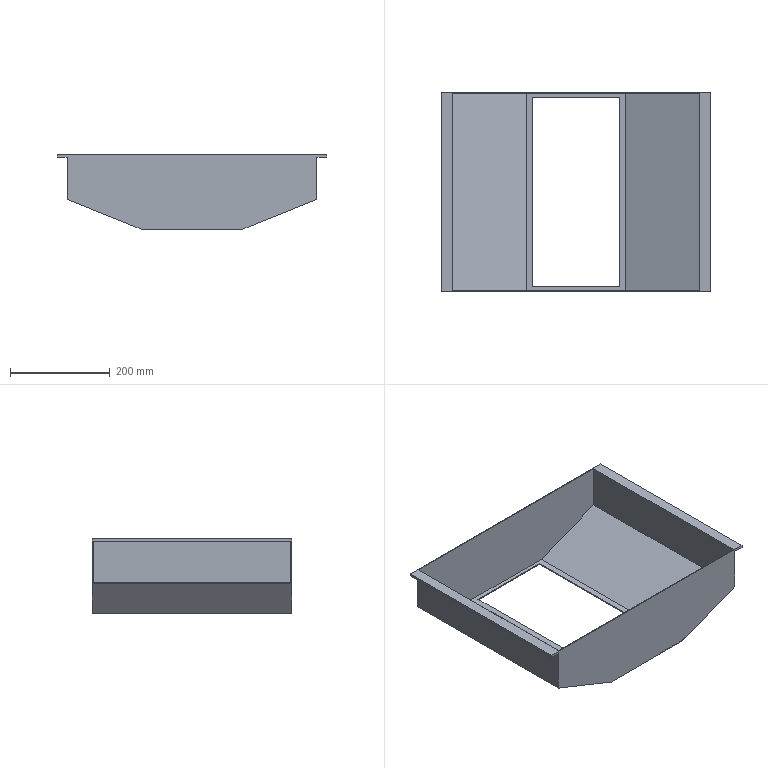Part | SolidWorks | features ICE 3, Extrusion 1, Shell 1 | 1 solid | 23 faces | box 540 x 400 x 150 mm | volume 765108 mm3 | plane 23
STEP:
#1=CARTESIAN_POINT('',(-99.615,198.,2.));
#2=VERTEX_POINT('',#1);
#3=CARTESIAN_POINT('',(-99.615,-198.,2.));
#4=VERTEX_POINT('',#3);
#5=CARTESIAN_POINT('',(-99.615,0.,2.));
#6=DIRECTION('',(0.,-1.,0.));
#7=VECTOR('',#6,1000.);
#8=LINE('',#5,#7);
#9=EDGE_CURVE('',#2,#4,#8,.T.);
#10=ORIENTED_EDGE('',*,*,#9,.T.);
#11=CARTESIAN_POINT('',(99.615,-198.,2.));
#12=VERTEX_POINT('',#11);
#13=CARTESIAN_POINT('',(0.,-198.,2.));
#14=DIRECTION('',(1.,0.,0.));
#15=VECTOR('',#14,1000.);
#16=LINE('',#13,#15);
#17=EDGE_CURVE('',#4,#12,#16,.T.);
#18=ORIENTED_EDGE('',*,*,#17,.T.);
#19=CARTESIAN_POINT('',(99.615,198.,2.));
#20=VERTEX_POINT('',#19);
#21=CARTESIAN_POINT('',(99.615,200.,2.));
#22=DIRECTION('',(0.,-1.,0.));
#23=VECTOR('',#22,1000.);
#24=LINE('',#21,#23);
#25=EDGE_CURVE('',#20,#12,#24,.T.);
#26=ORIENTED_EDGE('',*,*,#25,.F.);
#27=CARTESIAN_POINT('',(0.,198.,2.));
#28=DIRECTION('',(-1.,0.,0.));
#29=VECTOR('',#28,1000.);
#30=LINE('',#27,#29);
#31=EDGE_CURVE('',#20,#2,#30,.T.);
#32=ORIENTED_EDGE('',*,*,#31,.T.);
#33=EDGE_LOOP('',(#10,#18,#26,#32));
#34=FACE_OUTER_BOUND('',#33,.T.);
#35=CARTESIAN_POINT('',(87.5,-190.,2.));
#36=VERTEX_POINT('',#35);
#37=CARTESIAN_POINT('',(87.5,190.,2.));
#38=VERTEX_POINT('',#37);
#39=CARTESIAN_POINT('',(87.5,-190.,2.));
#40=DIRECTION('',(0.,1.,0.));
#41=VECTOR('',#40,1000.);
#42=LINE('',#39,#41);
#43=EDGE_CURVE('',#36,#38,#42,.T.);
#44=ORIENTED_EDGE('',*,*,#43,.F.);
#45=CARTESIAN_POINT('',(-87.5,-190.,2.));
#46=VERTEX_POINT('',#45);
#47=CARTESIAN_POINT('',(-87.5,-190.,2.));
#48=DIRECTION('',(1.,0.,0.));
#49=VECTOR('',#48,1000.);
#50=LINE('',#47,#49);
#51=EDGE_CURVE('',#46,#36,#50,.T.);
#52=ORIENTED_EDGE('',*,*,#51,.F.);
#53=CARTESIAN_POINT('',(-87.5,190.,2.));
#54=VERTEX_POINT('',#53);
#55=CARTESIAN_POINT('',(-87.5,-190.,2.));
#56=DIRECTION('',(0.,-1.,0.));
#57=VECTOR('',#56,1000.);
#58=LINE('',#55,#57);
#59=EDGE_CURVE('',#54,#46,#58,.T.);
#60=ORIENTED_EDGE('',*,*,#59,.F.);
#61=CARTESIAN_POINT('',(-87.5,190.,2.));
#62=DIRECTION('',(-1.,0.,0.));
#63=VECTOR('',#62,1000.);
#64=LINE('',#61,#63);
#65=EDGE_CURVE('',#38,#54,#64,.T.);
#66=ORIENTED_EDGE('',*,*,#65,.F.);
#67=EDGE_LOOP('',(#44,#52,#60,#66));
#68=FACE_BOUND('',#67,.T.);
#69=CARTESIAN_POINT('',(0.,0.,2.));
#70=DIRECTION('',(0.,0.,-1.));
#71=DIRECTION('',(-1.,0.,0.));
#72=AXIS2_PLACEMENT_3D('',#69,#70,#71);
#73=PLANE('',#72);
#74=ADVANCED_FACE('',(#34,#68),#73,.F.);
#75=CARTESIAN_POINT('',(-270.,-200.,150.));
#76=VERTEX_POINT('',#75);
#77=CARTESIAN_POINT('',(270.,-200.,150.));
#78=VERTEX_POINT('',#77);
#79=CARTESIAN_POINT('',(-250.,-200.,150.));
#80=DIRECTION('',(1.,0.,0.));
#81=VECTOR('',#80,1000.);
#82=LINE('',#79,#81);
#83=EDGE_CURVE('',#76,#78,#82,.T.);
#84=ORIENTED_EDGE('',*,*,#83,.T.);
#85=CARTESIAN_POINT('',(270.,200.,150.));
#86=VERTEX_POINT('',#85);
#87=CARTESIAN_POINT('',(270.,200.,150.));
#88=DIRECTION('',(0.,1.,0.));
#89=VECTOR('',#88,1000.);
#90=LINE('',#87,#89);
#91=EDGE_CURVE('',#78,#86,#90,.T.);
#92=ORIENTED_EDGE('',*,*,#91,.T.);
#93=CARTESIAN_POINT('',(-270.,200.,150.));
#94=VERTEX_POINT('',#93);
#95=CARTESIAN_POINT('',(-250.,200.,150.));
#96=DIRECTION('',(-1.,0.,0.));
#97=VECTOR('',#96,1000.);
#98=LINE('',#95,#97);
#99=EDGE_CURVE('',#86,#94,#98,.T.);
#100=ORIENTED_EDGE('',*,*,#99,.T.);
#101=CARTESIAN_POINT('',(-270.,200.,150.));
#102=DIRECTION('',(0.,-1.,0.));
#103=VECTOR('',#102,1000.);
#104=LINE('',#101,#103);
#105=EDGE_CURVE('',#94,#76,#104,.T.);
#106=ORIENTED_EDGE('',*,*,#105,.T.);
#107=EDGE_LOOP('',(#84,#92,#100,#106));
#108=FACE_OUTER_BOUND('',#107,.T.);
#109=CARTESIAN_POINT('',(248.,-198.,150.));
#110=VERTEX_POINT('',#109);
#111=CARTESIAN_POINT('',(248.,198.,150.));
#112=VERTEX_POINT('',#111);
#113=CARTESIAN_POINT('',(248.,0.,150.));
#114=DIRECTION('',(0.,1.,0.));
#115=VECTOR('',#114,1000.);
#116=LINE('',#113,#115);
#117=EDGE_CURVE('',#110,#112,#116,.T.);
#118=ORIENTED_EDGE('',*,*,#117,.F.);
#119=CARTESIAN_POINT('',(-248.,-198.,150.));
#120=VERTEX_POINT('',#119);
#121=CARTESIAN_POINT('',(0.,-198.,150.));
#122=DIRECTION('',(1.,0.,0.));
#123=VECTOR('',#122,1000.);
#124=LINE('',#121,#123);
#125=EDGE_CURVE('',#120,#110,#124,.T.);
#126=ORIENTED_EDGE('',*,*,#125,.F.);
#127=CARTESIAN_POINT('',(-248.,198.,150.));
#128=VERTEX_POINT('',#127);
#129=CARTESIAN_POINT('',(-248.,0.,150.));
#130=DIRECTION('',(0.,-1.,0.));
#131=VECTOR('',#130,1000.);
#132=LINE('',#129,#131);
#133=EDGE_CURVE('',#128,#120,#132,.T.);
#134=ORIENTED_EDGE('',*,*,#133,.F.);
#135=CARTESIAN_POINT('',(0.,198.,150.));
#136=DIRECTION('',(-1.,0.,0.));
#137=VECTOR('',#136,1000.);
#138=LINE('',#135,#137);
#139=EDGE_CURVE('',#112,#128,#138,.T.);
#140=ORIENTED_EDGE('',*,*,#139,.F.);
#141=EDGE_LOOP('',(#118,#126,#134,#140));
#142=FACE_BOUND('',#141,.T.);
#143=CARTESIAN_POINT('',(0.,0.,150.));
#144=DIRECTION('',(0.,0.,-1.));
#145=DIRECTION('',(-1.,0.,0.));
#146=AXIS2_PLACEMENT_3D('',#143,#144,#145);
#147=PLANE('',#146);
#148=ADVANCED_FACE('',(#108,#142),#147,.F.);
#149=CARTESIAN_POINT('',(250.,200.,145.));
#150=VERTEX_POINT('',#149);
#151=CARTESIAN_POINT('',(250.,200.,60.));
#152=VERTEX_POINT('',#151);
#153=CARTESIAN_POINT('',(250.,200.,150.));
#154=DIRECTION('',(0.,0.,-1.));
#155=VECTOR('',#154,1000.);
#156=LINE('',#153,#155);
#157=EDGE_CURVE('',#150,#152,#156,.T.);
#158=ORIENTED_EDGE('',*,*,#157,.F.);
#159=CARTESIAN_POINT('',(250.,-200.,145.));
#160=VERTEX_POINT('',#159);
#161=CARTESIAN_POINT('',(250.,200.,145.));
#162=DIRECTION('',(0.,-1.,0.));
#163=VECTOR('',#162,1000.);
#164=LINE('',#161,#163);
#165=EDGE_CURVE('',#150,#160,#164,.T.);
#166=ORIENTED_EDGE('',*,*,#165,.T.);
#167=CARTESIAN_POINT('',(250.,-200.,60.));
#168=VERTEX_POINT('',#167);
#169=CARTESIAN_POINT('',(250.,-200.,150.));
#170=DIRECTION('',(0.,0.,-1.));
#171=VECTOR('',#170,1000.);
#172=LINE('',#169,#171);
#173=EDGE_CURVE('',#160,#168,#172,.T.);
#174=ORIENTED_EDGE('',*,*,#173,.T.);
#175=CARTESIAN_POINT('',(250.,200.,60.));
#176=DIRECTION('',(0.,-1.,0.));
#177=VECTOR('',#176,1000.);
#178=LINE('',#175,#177);
#179=EDGE_CURVE('',#152,#168,#178,.T.);
#180=ORIENTED_EDGE('',*,*,#179,.F.);
#181=EDGE_LOOP('',(#158,#166,#174,#180));
#182=FACE_OUTER_BOUND('',#181,.T.);
#183=CARTESIAN_POINT('',(250.,-200.,150.));
#184=DIRECTION('',(-1.,0.,0.));
#185=DIRECTION('',(0.,0.,1.));
#186=AXIS2_PLACEMENT_3D('',#183,#184,#185);
#187=PLANE('',#186);
#188=ADVANCED_FACE('',(#182),#187,.F.);
#189=CARTESIAN_POINT('',(100.,200.,0.));
#190=VERTEX_POINT('',#189);
#191=CARTESIAN_POINT('',(-100.,200.,0.));
#192=VERTEX_POINT('',#191);
#193=CARTESIAN_POINT('',(-250.,200.,0.));
#194=DIRECTION('',(-1.,0.,0.));
#195=VECTOR('',#194,1000.);
#196=LINE('',#193,#195);
#197=EDGE_CURVE('',#190,#192,#196,.T.);
#198=ORIENTED_EDGE('',*,*,#197,.T.);
#199=CARTESIAN_POINT('',(-250.,200.,60.));
#200=VERTEX_POINT('',#199);
#201=CARTESIAN_POINT('',(-100.,200.,0.));
#202=DIRECTION('',(-0.9285,0.,0.3714));
#203=VECTOR('',#202,1000.);
#204=LINE('',#201,#203);
#205=EDGE_CURVE('',#192,#200,#204,.T.);
#206=ORIENTED_EDGE('',*,*,#205,.T.);
#207=CARTESIAN_POINT('',(-250.,200.,145.));
#208=VERTEX_POINT('',#207);
#209=CARTESIAN_POINT('',(-250.,200.,150.));
#210=DIRECTION('',(0.,0.,-1.));
#211=VECTOR('',#210,1000.);
#212=LINE('',#209,#211);
#213=EDGE_CURVE('',#208,#200,#212,.T.);
#214=ORIENTED_EDGE('',*,*,#213,.F.);
#215=CARTESIAN_POINT('',(-270.,200.,145.));
#216=VERTEX_POINT('',#215);
#217=CARTESIAN_POINT('',(-250.,200.,145.));
#218=DIRECTION('',(-1.,0.,0.));
#219=VECTOR('',#218,1000.);
#220=LINE('',#217,#219);
#221=EDGE_CURVE('',#208,#216,#220,.T.);
#222=ORIENTED_EDGE('',*,*,#221,.T.);
#223=CARTESIAN_POINT('',(-270.,200.,145.));
#224=DIRECTION('',(0.,0.,1.));
#225=VECTOR('',#224,1000.);
#226=LINE('',#223,#225);
#227=EDGE_CURVE('',#216,#94,#226,.T.);
#228=ORIENTED_EDGE('',*,*,#227,.T.);
#229=ORIENTED_EDGE('',*,*,#99,.F.);
#230=CARTESIAN_POINT('',(270.,200.,145.));
#231=VERTEX_POINT('',#230);
#232=CARTESIAN_POINT('',(270.,200.,145.));
#233=DIRECTION('',(0.,0.,1.));
#234=VECTOR('',#233,1000.);
#235=LINE('',#232,#234);
#236=EDGE_CURVE('',#231,#86,#235,.T.);
#237=ORIENTED_EDGE('',*,*,#236,.F.);
#238=CARTESIAN_POINT('',(250.,200.,145.));
#239=DIRECTION('',(-1.,0.,0.));
#240=VECTOR('',#239,1000.);
#241=LINE('',#238,#240);
#242=EDGE_CURVE('',#231,#150,#241,.T.);
#243=ORIENTED_EDGE('',*,*,#242,.T.);
#244=ORIENTED_EDGE('',*,*,#157,.T.);
#245=CARTESIAN_POINT('',(250.,200.,60.));
#246=DIRECTION('',(-0.9285,0.,-0.3714));
#247=VECTOR('',#246,1000.);
#248=LINE('',#245,#247);
#249=EDGE_CURVE('',#152,#190,#248,.T.);
#250=ORIENTED_EDGE('',*,*,#249,.T.);
#251=EDGE_LOOP('',(#198,#206,#214,#222,#228,#229,#237,#243,#244,#250));
#252=FACE_OUTER_BOUND('',#251,.T.);
#253=CARTESIAN_POINT('',(-250.,200.,150.));
#254=DIRECTION('',(0.,-1.,0.));
#255=DIRECTION('',(0.,0.,-1.));
#256=AXIS2_PLACEMENT_3D('',#253,#254,#255);
#257=PLANE('',#256);
#258=ADVANCED_FACE('',(#252),#257,.F.);
#259=CARTESIAN_POINT('',(-250.,-200.,145.));
#260=VERTEX_POINT('',#259);
#261=CARTESIAN_POINT('',(-250.,-200.,60.));
#262=VERTEX_POINT('',#261);
#263=CARTESIAN_POINT('',(-250.,-200.,150.));
#264=DIRECTION('',(0.,0.,-1.));
#265=VECTOR('',#264,1000.);
#266=LINE('',#263,#265);
#267=EDGE_CURVE('',#260,#262,#266,.T.);
#268=ORIENTED_EDGE('',*,*,#267,.F.);
#269=CARTESIAN_POINT('',(-250.,200.,145.));
#270=DIRECTION('',(0.,1.,0.));
#271=VECTOR('',#270,1000.);
#272=LINE('',#269,#271);
#273=EDGE_CURVE('',#260,#208,#272,.T.);
#274=ORIENTED_EDGE('',*,*,#273,.T.);
#275=ORIENTED_EDGE('',*,*,#213,.T.);
#276=CARTESIAN_POINT('',(-250.,200.,60.));
#277=DIRECTION('',(0.,-1.,0.));
#278=VECTOR('',#277,1000.);
#279=LINE('',#276,#278);
#280=EDGE_CURVE('',#200,#262,#279,.T.);
#281=ORIENTED_EDGE('',*,*,#280,.T.);
#282=EDGE_LOOP('',(#268,#274,#275,#281));
#283=FACE_OUTER_BOUND('',#282,.T.);
#284=CARTESIAN_POINT('',(-250.,-200.,150.));
#285=DIRECTION('',(1.,0.,0.));
#286=DIRECTION('',(0.,0.,-1.));
#287=AXIS2_PLACEMENT_3D('',#284,#285,#286);
#288=PLANE('',#287);
#289=ADVANCED_FACE('',(#283),#288,.F.);
#290=ORIENTED_EDGE('',*,*,#83,.F.);
#291=CARTESIAN_POINT('',(-270.,-200.,145.));
#292=VERTEX_POINT('',#291);
#293=CARTESIAN_POINT('',(-270.,-200.,145.));
#294=DIRECTION('',(0.,0.,1.));
#295=VECTOR('',#294,1000.);
#296=LINE('',#293,#295);
#297=EDGE_CURVE('',#292,#76,#296,.T.);
#298=ORIENTED_EDGE('',*,*,#297,.F.);
#299=CARTESIAN_POINT('',(-250.,-200.,145.));
#300=DIRECTION('',(1.,0.,0.));
#301=VECTOR('',#300,1000.);
#302=LINE('',#299,#301);
#303=EDGE_CURVE('',#292,#260,#302,.T.);
#304=ORIENTED_EDGE('',*,*,#303,.T.);
#305=ORIENTED_EDGE('',*,*,#267,.T.);
#306=CARTESIAN_POINT('',(-100.,-200.,0.));
#307=VERTEX_POINT('',#306);
#308=CARTESIAN_POINT('',(-100.,-200.,0.));
#309=DIRECTION('',(-0.9285,0.,0.3714));
#310=VECTOR('',#309,1000.);
#311=LINE('',#308,#310);
#312=EDGE_CURVE('',#307,#262,#311,.T.);
#313=ORIENTED_EDGE('',*,*,#312,.F.);
#314=CARTESIAN_POINT('',(100.,-200.,0.));
#315=VERTEX_POINT('',#314);
#316=CARTESIAN_POINT('',(-250.,-200.,0.));
#317=DIRECTION('',(1.,0.,0.));
#318=VECTOR('',#317,1000.);
#319=LINE('',#316,#318);
#320=EDGE_CURVE('',#307,#315,#319,.T.);
#321=ORIENTED_EDGE('',*,*,#320,.T.);
#322=CARTESIAN_POINT('',(250.,-200.,60.));
#323=DIRECTION('',(-0.9285,0.,-0.3714));
#324=VECTOR('',#323,1000.);
#325=LINE('',#322,#324);
#326=EDGE_CURVE('',#168,#315,#325,.T.);
#327=ORIENTED_EDGE('',*,*,#326,.F.);
#328=ORIENTED_EDGE('',*,*,#173,.F.);
#329=CARTESIAN_POINT('',(270.,-200.,145.));
#330=VERTEX_POINT('',#329);
#331=CARTESIAN_POINT('',(250.,-200.,145.));
#332=DIRECTION('',(1.,0.,0.));
#333=VECTOR('',#332,1000.);
#334=LINE('',#331,#333);
#335=EDGE_CURVE('',#160,#330,#334,.T.);
#336=ORIENTED_EDGE('',*,*,#335,.T.);
#337=CARTESIAN_POINT('',(270.,-200.,145.));
#338=DIRECTION('',(0.,0.,1.));
#339=VECTOR('',#338,1000.);
#340=LINE('',#337,#339);
#341=EDGE_CURVE('',#330,#78,#340,.T.);
#342=ORIENTED_EDGE('',*,*,#341,.T.);
#343=EDGE_LOOP('',(#290,#298,#304,#305,#313,#321,#327,#328,#336,#342));
#344=FACE_OUTER_BOUND('',#343,.T.);
#345=CARTESIAN_POINT('',(-250.,-200.,150.));
#346=DIRECTION('',(0.,1.,0.));
#347=DIRECTION('',(0.,0.,1.));
#348=AXIS2_PLACEMENT_3D('',#345,#346,#347);
#349=PLANE('',#348);
#350=ADVANCED_FACE('',(#344),#349,.F.);
#351=CARTESIAN_POINT('',(87.5,-190.,0.));
#352=VERTEX_POINT('',#351);
#353=CARTESIAN_POINT('',(87.5,190.,0.));
#354=VERTEX_POINT('',#353);
#355=CARTESIAN_POINT('',(87.5,-190.,0.));
#356=DIRECTION('',(0.,1.,0.));
#357=VECTOR('',#356,1000.);
#358=LINE('',#355,#357);
#359=EDGE_CURVE('',#352,#354,#358,.T.);
#360=ORIENTED_EDGE('',*,*,#359,.T.);
#361=CARTESIAN_POINT('',(-87.5,190.,0.));
#362=VERTEX_POINT('',#361);
#363=CARTESIAN_POINT('',(-87.5,190.,0.));
#364=DIRECTION('',(-1.,0.,0.));
#365=VECTOR('',#364,1000.);
#366=LINE('',#363,#365);
#367=EDGE_CURVE('',#354,#362,#366,.T.);
#368=ORIENTED_EDGE('',*,*,#367,.T.);
#369=CARTESIAN_POINT('',(-87.5,-190.,0.));
#370=VERTEX_POINT('',#369);
#371=CARTESIAN_POINT('',(-87.5,-190.,0.));
#372=DIRECTION('',(0.,-1.,0.));
#373=VECTOR('',#372,1000.);
#374=LINE('',#371,#373);
#375=EDGE_CURVE('',#362,#370,#374,.T.);
#376=ORIENTED_EDGE('',*,*,#375,.T.);
#377=CARTESIAN_POINT('',(-87.5,-190.,0.));
#378=DIRECTION('',(1.,0.,0.));
#379=VECTOR('',#378,1000.);
#380=LINE('',#377,#379);
#381=EDGE_CURVE('',#370,#352,#380,.T.);
#382=ORIENTED_EDGE('',*,*,#381,.T.);
#383=EDGE_LOOP('',(#360,#368,#376,#382));
#384=FACE_BOUND('',#383,.T.);
#385=CARTESIAN_POINT('',(-100.,200.,0.));
#386=DIRECTION('',(0.,-1.,0.));
#387=VECTOR('',#386,1000.);
#388=LINE('',#385,#387);
#389=EDGE_CURVE('',#192,#307,#388,.T.);
#390=ORIENTED_EDGE('',*,*,#389,.F.);
#391=ORIENTED_EDGE('',*,*,#197,.F.);
#392=CARTESIAN_POINT('',(100.,200.,0.));
#393=DIRECTION('',(0.,-1.,0.));
#394=VECTOR('',#393,1000.);
#395=LINE('',#392,#394);
#396=EDGE_CURVE('',#190,#315,#395,.T.);
#397=ORIENTED_EDGE('',*,*,#396,.T.);
#398=ORIENTED_EDGE('',*,*,#320,.F.);
#399=EDGE_LOOP('',(#390,#391,#397,#398));
#400=FACE_OUTER_BOUND('',#399,.T.);
#401=CARTESIAN_POINT('',(0.,0.,0.));
#402=DIRECTION('',(0.,0.,-1.));
#403=DIRECTION('',(-1.,0.,0.));
#404=AXIS2_PLACEMENT_3D('',#401,#402,#403);
#405=PLANE('',#404);
#406=ADVANCED_FACE('',(#384,#400),#405,.T.);
#407=ORIENTED_EDGE('',*,*,#326,.T.);
#408=ORIENTED_EDGE('',*,*,#396,.F.);
#409=ORIENTED_EDGE('',*,*,#249,.F.);
#410=ORIENTED_EDGE('',*,*,#179,.T.);
#411=EDGE_LOOP('',(#407,#408,#409,#410));
#412=FACE_OUTER_BOUND('',#411,.T.);
#413=CARTESIAN_POINT('',(250.,200.,60.));
#414=DIRECTION('',(-0.3714,0.,0.9285));
#415=DIRECTION('',(0.9285,0.,0.3714));
#416=AXIS2_PLACEMENT_3D('',#413,#414,#415);
#417=PLANE('',#416);
#418=ADVANCED_FACE('',(#412),#417,.F.);
#419=ORIENTED_EDGE('',*,*,#312,.T.);
#420=ORIENTED_EDGE('',*,*,#280,.F.);
#421=ORIENTED_EDGE('',*,*,#205,.F.);
#422=ORIENTED_EDGE('',*,*,#389,.T.);
#423=EDGE_LOOP('',(#419,#420,#421,#422));
#424=FACE_OUTER_BOUND('',#423,.T.);
#425=CARTESIAN_POINT('',(-100.,200.,0.));
#426=DIRECTION('',(0.3714,0.,0.9285));
#427=DIRECTION('',(0.9285,0.,-0.3714));
#428=AXIS2_PLACEMENT_3D('',#425,#426,#427);
#429=PLANE('',#428);
#430=ADVANCED_FACE('',(#424),#429,.F.);
#431=CARTESIAN_POINT('',(248.,-198.,61.354));
#432=VERTEX_POINT('',#431);
#433=CARTESIAN_POINT('',(248.,-198.,150.));
#434=DIRECTION('',(0.,0.,-1.));
#435=VECTOR('',#434,1000.);
#436=LINE('',#433,#435);
#437=EDGE_CURVE('',#110,#432,#436,.T.);
#438=ORIENTED_EDGE('',*,*,#437,.F.);
#439=ORIENTED_EDGE('',*,*,#117,.T.);
#440=CARTESIAN_POINT('',(248.,198.,61.354));
#441=VERTEX_POINT('',#440);
#442=CARTESIAN_POINT('',(248.,198.,150.));
#443=DIRECTION('',(0.,0.,-1.));
#444=VECTOR('',#443,1000.);
#445=LINE('',#442,#444);
#446=EDGE_CURVE('',#112,#441,#445,.T.);
#447=ORIENTED_EDGE('',*,*,#446,.T.);
#448=CARTESIAN_POINT('',(248.,200.,61.354));
#449=DIRECTION('',(0.,-1.,0.));
#450=VECTOR('',#449,1000.);
#451=LINE('',#448,#450);
#452=EDGE_CURVE('',#441,#432,#451,.T.);
#453=ORIENTED_EDGE('',*,*,#452,.T.);
#454=EDGE_LOOP('',(#438,#439,#447,#453));
#455=FACE_OUTER_BOUND('',#454,.T.);
#456=CARTESIAN_POINT('',(248.,-200.,150.));
#457=DIRECTION('',(-1.,0.,0.));
#458=DIRECTION('',(0.,0.,1.));
#459=AXIS2_PLACEMENT_3D('',#456,#457,#458);
#460=PLANE('',#459);
#461=ADVANCED_FACE('',(#455),#460,.T.);
#462=ORIENTED_EDGE('',*,*,#31,.F.);
#463=CARTESIAN_POINT('',(-150.743,198.,-98.143));
#464=DIRECTION('',(-0.9285,0.,-0.3714));
#465=VECTOR('',#464,1000.);
#466=LINE('',#463,#465);
#467=EDGE_CURVE('',#441,#20,#466,.T.);
#468=ORIENTED_EDGE('',*,*,#467,.F.);
#469=ORIENTED_EDGE('',*,*,#446,.F.);
#470=ORIENTED_EDGE('',*,*,#139,.T.);
#471=CARTESIAN_POINT('',(-248.,198.,61.354));
#472=VERTEX_POINT('',#471);
#473=CARTESIAN_POINT('',(-248.,198.,150.));
#474=DIRECTION('',(0.,0.,-1.));
#475=VECTOR('',#474,1000.);
#476=LINE('',#473,#475);
#477=EDGE_CURVE('',#128,#472,#476,.T.);
#478=ORIENTED_EDGE('',*,*,#477,.T.);
#479=CARTESIAN_POINT('',(-280.292,198.,74.271));
#480=DIRECTION('',(-0.9285,0.,0.3714));
#481=VECTOR('',#480,1000.);
#482=LINE('',#479,#481);
#483=EDGE_CURVE('',#2,#472,#482,.T.);
#484=ORIENTED_EDGE('',*,*,#483,.F.);
#485=EDGE_LOOP('',(#462,#468,#469,#470,#478,#484));
#486=FACE_OUTER_BOUND('',#485,.T.);
#487=CARTESIAN_POINT('',(-250.,198.,150.));
#488=DIRECTION('',(0.,-1.,0.));
#489=DIRECTION('',(0.,0.,-1.));
#490=AXIS2_PLACEMENT_3D('',#487,#488,#489);
#491=PLANE('',#490);
#492=ADVANCED_FACE('',(#486),#491,.T.);
#493=ORIENTED_EDGE('',*,*,#477,.F.);
#494=ORIENTED_EDGE('',*,*,#133,.T.);
#495=CARTESIAN_POINT('',(-248.,-198.,61.354));
#496=VERTEX_POINT('',#495);
#497=CARTESIAN_POINT('',(-248.,-198.,150.));
#498=DIRECTION('',(0.,0.,-1.));
#499=VECTOR('',#498,1000.);
#500=LINE('',#497,#499);
#501=EDGE_CURVE('',#120,#496,#500,.T.);
#502=ORIENTED_EDGE('',*,*,#501,.T.);
#503=CARTESIAN_POINT('',(-248.,-200.,61.354));
#504=DIRECTION('',(0.,-1.,0.));
#505=VECTOR('',#504,1000.);
#506=LINE('',#503,#505);
#507=EDGE_CURVE('',#472,#496,#506,.T.);
#508=ORIENTED_EDGE('',*,*,#507,.F.);
#509=EDGE_LOOP('',(#493,#494,#502,#508));
#510=FACE_OUTER_BOUND('',#509,.T.);
#511=CARTESIAN_POINT('',(-248.,-200.,150.));
#512=DIRECTION('',(1.,0.,0.));
#513=DIRECTION('',(0.,0.,-1.));
#514=AXIS2_PLACEMENT_3D('',#511,#512,#513);
#515=PLANE('',#514);
#516=ADVANCED_FACE('',(#510),#515,.T.);
#517=ORIENTED_EDGE('',*,*,#501,.F.);
#518=ORIENTED_EDGE('',*,*,#125,.T.);
#519=ORIENTED_EDGE('',*,*,#437,.T.);
#520=CARTESIAN_POINT('',(249.257,-198.,61.857));
#521=DIRECTION('',(-0.9285,0.,-0.3714));
#522=VECTOR('',#521,1000.);
#523=LINE('',#520,#522);
#524=EDGE_CURVE('',#432,#12,#523,.T.);
#525=ORIENTED_EDGE('',*,*,#524,.T.);
#526=ORIENTED_EDGE('',*,*,#17,.F.);
#527=CARTESIAN_POINT('',(-99.257,-198.,1.857));
#528=DIRECTION('',(-0.9285,0.,0.3714));
#529=VECTOR('',#528,1000.);
#530=LINE('',#527,#529);
#531=EDGE_CURVE('',#4,#496,#530,.T.);
#532=ORIENTED_EDGE('',*,*,#531,.T.);
#533=EDGE_LOOP('',(#517,#518,#519,#525,#526,#532));
#534=FACE_OUTER_BOUND('',#533,.T.);
#535=CARTESIAN_POINT('',(-250.,-198.,150.));
#536=DIRECTION('',(0.,1.,0.));
#537=DIRECTION('',(0.,0.,1.));
#538=AXIS2_PLACEMENT_3D('',#535,#536,#537);
#539=PLANE('',#538);
#540=ADVANCED_FACE('',(#534),#539,.T.);
#541=ORIENTED_EDGE('',*,*,#524,.F.);
#542=ORIENTED_EDGE('',*,*,#452,.F.);
#543=ORIENTED_EDGE('',*,*,#467,.T.);
#544=ORIENTED_EDGE('',*,*,#25,.T.);
#545=EDGE_LOOP('',(#541,#542,#543,#544));
#546=FACE_OUTER_BOUND('',#545,.T.);
#547=CARTESIAN_POINT('',(249.257,200.,61.857));
#548=DIRECTION('',(-0.3714,0.,0.9285));
#549=DIRECTION('',(0.9285,0.,0.3714));
#550=AXIS2_PLACEMENT_3D('',#547,#548,#549);
#551=PLANE('',#550);
#552=ADVANCED_FACE('',(#546),#551,.T.);
#553=ORIENTED_EDGE('',*,*,#531,.F.);
#554=ORIENTED_EDGE('',*,*,#9,.F.);
#555=ORIENTED_EDGE('',*,*,#483,.T.);
#556=ORIENTED_EDGE('',*,*,#507,.T.);
#557=EDGE_LOOP('',(#553,#554,#555,#556));
#558=FACE_OUTER_BOUND('',#557,.T.);
#559=CARTESIAN_POINT('',(-99.257,200.,1.857));
#560=DIRECTION('',(0.3714,0.,0.9285));
#561=DIRECTION('',(0.9285,0.,-0.3714));
#562=AXIS2_PLACEMENT_3D('',#559,#560,#561);
#563=PLANE('',#562);
#564=ADVANCED_FACE('',(#558),#563,.T.);
#565=ORIENTED_EDGE('',*,*,#105,.F.);
#566=ORIENTED_EDGE('',*,*,#227,.F.);
#567=CARTESIAN_POINT('',(-270.,200.,145.));
#568=DIRECTION('',(0.,-1.,0.));
#569=VECTOR('',#568,1000.);
#570=LINE('',#567,#569);
#571=EDGE_CURVE('',#216,#292,#570,.T.);
#572=ORIENTED_EDGE('',*,*,#571,.T.);
#573=ORIENTED_EDGE('',*,*,#297,.T.);
#574=EDGE_LOOP('',(#565,#566,#572,#573));
#575=FACE_OUTER_BOUND('',#574,.T.);
#576=CARTESIAN_POINT('',(-270.,200.,145.));
#577=DIRECTION('',(-1.,0.,0.));
#578=DIRECTION('',(0.,0.,1.));
#579=AXIS2_PLACEMENT_3D('',#576,#577,#578);
#580=PLANE('',#579);
#581=ADVANCED_FACE('',(#575),#580,.T.);
#582=ORIENTED_EDGE('',*,*,#273,.F.);
#583=ORIENTED_EDGE('',*,*,#303,.F.);
#584=ORIENTED_EDGE('',*,*,#571,.F.);
#585=ORIENTED_EDGE('',*,*,#221,.F.);
#586=EDGE_LOOP('',(#582,#583,#584,#585));
#587=FACE_OUTER_BOUND('',#586,.T.);
#588=CARTESIAN_POINT('',(0.,0.,145.));
#589=DIRECTION('',(0.,0.,-1.));
#590=DIRECTION('',(-1.,0.,0.));
#591=AXIS2_PLACEMENT_3D('',#588,#589,#590);
#592=PLANE('',#591);
#593=ADVANCED_FACE('',(#587),#592,.T.);
#594=ORIENTED_EDGE('',*,*,#91,.F.);
#595=ORIENTED_EDGE('',*,*,#341,.F.);
#596=CARTESIAN_POINT('',(270.,200.,145.));
#597=DIRECTION('',(0.,1.,0.));
#598=VECTOR('',#597,1000.);
#599=LINE('',#596,#598);
#600=EDGE_CURVE('',#330,#231,#599,.T.);
#601=ORIENTED_EDGE('',*,*,#600,.T.);
#602=ORIENTED_EDGE('',*,*,#236,.T.);
#603=EDGE_LOOP('',(#594,#595,#601,#602));
#604=FACE_OUTER_BOUND('',#603,.T.);
#605=CARTESIAN_POINT('',(270.,200.,145.));
#606=DIRECTION('',(1.,0.,0.));
#607=DIRECTION('',(0.,1.,0.));
#608=AXIS2_PLACEMENT_3D('',#605,#606,#607);
#609=PLANE('',#608);
#610=ADVANCED_FACE('',(#604),#609,.T.);
#611=ORIENTED_EDGE('',*,*,#165,.F.);
#612=ORIENTED_EDGE('',*,*,#242,.F.);
#613=ORIENTED_EDGE('',*,*,#600,.F.);
#614=ORIENTED_EDGE('',*,*,#335,.F.);
#615=EDGE_LOOP('',(#611,#612,#613,#614));
#616=FACE_OUTER_BOUND('',#615,.T.);
#617=CARTESIAN_POINT('',(0.,0.,145.));
#618=DIRECTION('',(0.,0.,1.));
#619=DIRECTION('',(1.,0.,0.));
#620=AXIS2_PLACEMENT_3D('',#617,#618,#619);
#621=PLANE('',#620);
#622=ADVANCED_FACE('',(#616),#621,.F.);
#623=ORIENTED_EDGE('',*,*,#43,.T.);
#624=CARTESIAN_POINT('',(87.5,190.,0.));
#625=DIRECTION('',(0.,0.,1.));
#626=VECTOR('',#625,1000.);
#627=LINE('',#624,#626);
#628=EDGE_CURVE('',#354,#38,#627,.T.);
#629=ORIENTED_EDGE('',*,*,#628,.F.);
#630=ORIENTED_EDGE('',*,*,#359,.F.);
#631=CARTESIAN_POINT('',(87.5,-190.,0.));
#632=DIRECTION('',(0.,0.,1.));
#633=VECTOR('',#632,1000.);
#634=LINE('',#631,#633);
#635=EDGE_CURVE('',#352,#36,#634,.T.);
#636=ORIENTED_EDGE('',*,*,#635,.T.);
#637=EDGE_LOOP('',(#623,#629,#630,#636));
#638=FACE_OUTER_BOUND('',#637,.T.);
#639=CARTESIAN_POINT('',(87.5,-190.,0.));
#640=DIRECTION('',(1.,0.,0.));
#641=DIRECTION('',(0.,0.,-1.));
#642=AXIS2_PLACEMENT_3D('',#639,#640,#641);
#643=PLANE('',#642);
#644=ADVANCED_FACE('',(#638),#643,.F.);
#645=ORIENTED_EDGE('',*,*,#51,.T.);
#646=ORIENTED_EDGE('',*,*,#635,.F.);
#647=ORIENTED_EDGE('',*,*,#381,.F.);
#648=CARTESIAN_POINT('',(-87.5,-190.,0.));
#649=DIRECTION('',(0.,0.,1.));
#650=VECTOR('',#649,1000.);
#651=LINE('',#648,#650);
#652=EDGE_CURVE('',#370,#46,#651,.T.);
#653=ORIENTED_EDGE('',*,*,#652,.T.);
#654=EDGE_LOOP('',(#645,#646,#647,#653));
#655=FACE_OUTER_BOUND('',#654,.T.);
#656=CARTESIAN_POINT('',(-87.5,-190.,0.));
#657=DIRECTION('',(0.,-1.,0.));
#658=DIRECTION('',(0.,0.,-1.));
#659=AXIS2_PLACEMENT_3D('',#656,#657,#658);
#660=PLANE('',#659);
#661=ADVANCED_FACE('',(#655),#660,.F.);
#662=ORIENTED_EDGE('',*,*,#59,.T.);
#663=ORIENTED_EDGE('',*,*,#652,.F.);
#664=ORIENTED_EDGE('',*,*,#375,.F.);
#665=CARTESIAN_POINT('',(-87.5,190.,0.));
#666=DIRECTION('',(0.,0.,1.));
#667=VECTOR('',#666,1000.);
#668=LINE('',#665,#667);
#669=EDGE_CURVE('',#362,#54,#668,.T.);
#670=ORIENTED_EDGE('',*,*,#669,.T.);
#671=EDGE_LOOP('',(#662,#663,#664,#670));
#672=FACE_OUTER_BOUND('',#671,.T.);
#673=CARTESIAN_POINT('',(-87.5,-190.,0.));
#674=DIRECTION('',(-1.,0.,0.));
#675=DIRECTION('',(0.,0.,1.));
#676=AXIS2_PLACEMENT_3D('',#673,#674,#675);
#677=PLANE('',#676);
#678=ADVANCED_FACE('',(#672),#677,.F.);
#679=ORIENTED_EDGE('',*,*,#65,.T.);
#680=ORIENTED_EDGE('',*,*,#669,.F.);
#681=ORIENTED_EDGE('',*,*,#367,.F.);
#682=ORIENTED_EDGE('',*,*,#628,.T.);
#683=EDGE_LOOP('',(#679,#680,#681,#682));
#684=FACE_OUTER_BOUND('',#683,.T.);
#685=CARTESIAN_POINT('',(-87.5,190.,0.));
#686=DIRECTION('',(0.,1.,0.));
#687=DIRECTION('',(0.,0.,1.));
#688=AXIS2_PLACEMENT_3D('',#685,#686,#687);
#689=PLANE('',#688);
#690=ADVANCED_FACE('',(#684),#689,.F.);
#691=CLOSED_SHELL('',(#74,#148,#188,#258,#289,#350,#406,#418,#430,#461,#492,#516,#540,#552,#564,#581,#593,#610,#622,#644,#661,#678,#690));
#692=MANIFOLD_SOLID_BREP('',#691);
#693=CARTESIAN_POINT('',(0.,0.,0.));
#694=DIRECTION('',(0.,0.,1.));
#695=DIRECTION('',(1.,0.,0.));
#696=AXIS2_PLACEMENT_3D('',#693,#694,#695);
#697=(LENGTH_UNIT()NAMED_UNIT(*)SI_UNIT(.MILLI.,.METRE.));
#698=UNCERTAINTY_MEASURE_WITH_UNIT(LENGTH_MEASURE(0.00001),#697,'','');
#699=(NAMED_UNIT(*)PLANE_ANGLE_UNIT()SI_UNIT($,.RADIAN.));
#700=(NAMED_UNIT(*)SI_UNIT($,.STERADIAN.)SOLID_ANGLE_UNIT());
#701=(GEOMETRIC_REPRESENTATION_CONTEXT(3)GLOBAL_UNCERTAINTY_ASSIGNED_CONTEXT((#698))GLOBAL_UNIT_ASSIGNED_CONTEXT((#697,#699,#700))REPRESENTATION_CONTEXT('',''));
#702=ADVANCED_BREP_SHAPE_REPRESENTATION('',(#692,#696),#701);